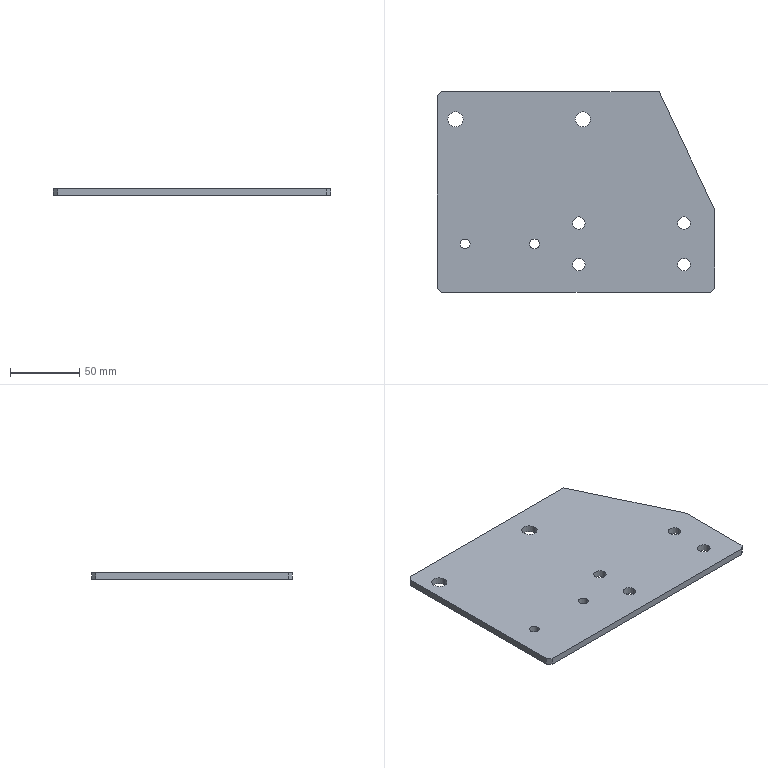Part | SolidWorks | features Extrusion 1 | 1 solid | 26 faces | box 200 x 145 x 5 mm | volume 133825 mm3 | cylinder 16 | plane 10 | commonest cylinder face diameters 9 x8 7 x4 11 x4
STEP:
#1=CARTESIAN_POINT('',(-92.5,52.5,-2.5));
#2=VERTEX_POINT('',#1);
#3=CARTESIAN_POINT('',(-81.5,52.5,-2.5));
#4=VERTEX_POINT('',#3);
#5=CARTESIAN_POINT('',(-87.,52.5,-2.5));
#6=DIRECTION('',(0.,0.,1.));
#7=DIRECTION('',(-1.,0.,0.));
#8=AXIS2_PLACEMENT_3D('',#5,#6,#7);
#9=CIRCLE('',#8,5.5);
#10=EDGE_CURVE('',#2,#4,#9,.T.);
#11=ORIENTED_EDGE('',*,*,#10,.F.);
#12=CARTESIAN_POINT('',(-92.5,52.5,2.5));
#13=VERTEX_POINT('',#12);
#14=CARTESIAN_POINT('',(-92.5,52.5,-2.5));
#15=DIRECTION('',(0.,0.,1.));
#16=VECTOR('',#15,1000.);
#17=LINE('',#14,#16);
#18=EDGE_CURVE('',#2,#13,#17,.T.);
#19=ORIENTED_EDGE('',*,*,#18,.T.);
#20=CARTESIAN_POINT('',(-81.5,52.5,2.5));
#21=VERTEX_POINT('',#20);
#22=CARTESIAN_POINT('',(-87.,52.5,2.5));
#23=DIRECTION('',(0.,0.,1.));
#24=DIRECTION('',(-1.,0.,0.));
#25=AXIS2_PLACEMENT_3D('',#22,#23,#24);
#26=CIRCLE('',#25,5.5);
#27=EDGE_CURVE('',#13,#21,#26,.T.);
#28=ORIENTED_EDGE('',*,*,#27,.T.);
#29=CARTESIAN_POINT('',(-81.5,52.5,-2.5));
#30=DIRECTION('',(0.,0.,1.));
#31=VECTOR('',#30,1000.);
#32=LINE('',#29,#31);
#33=EDGE_CURVE('',#4,#21,#32,.T.);
#34=ORIENTED_EDGE('',*,*,#33,.F.);
#35=EDGE_LOOP('',(#11,#19,#28,#34));
#36=FACE_OUTER_BOUND('',#35,.T.);
#37=CARTESIAN_POINT('',(-87.,52.5,-2.5));
#38=DIRECTION('',(0.,0.,1.));
#39=DIRECTION('',(1.,0.,0.));
#40=AXIS2_PLACEMENT_3D('',#37,#38,#39);
#41=CYLINDRICAL_SURFACE('',#40,5.5);
#42=ADVANCED_FACE('',(#36),#41,.F.);
#43=CARTESIAN_POINT('',(73.5,-22.5,-2.5));
#44=VERTEX_POINT('',#43);
#45=CARTESIAN_POINT('',(82.5,-22.5,-2.5));
#46=VERTEX_POINT('',#45);
#47=CARTESIAN_POINT('',(78.,-22.5,-2.5));
#48=DIRECTION('',(0.,0.,1.));
#49=DIRECTION('',(-1.,0.,0.));
#50=AXIS2_PLACEMENT_3D('',#47,#48,#49);
#51=CIRCLE('',#50,4.5);
#52=EDGE_CURVE('',#44,#46,#51,.T.);
#53=ORIENTED_EDGE('',*,*,#52,.F.);
#54=CARTESIAN_POINT('',(73.5,-22.5,2.5));
#55=VERTEX_POINT('',#54);
#56=CARTESIAN_POINT('',(73.5,-22.5,-2.5));
#57=DIRECTION('',(0.,0.,1.));
#58=VECTOR('',#57,1000.);
#59=LINE('',#56,#58);
#60=EDGE_CURVE('',#44,#55,#59,.T.);
#61=ORIENTED_EDGE('',*,*,#60,.T.);
#62=CARTESIAN_POINT('',(82.5,-22.5,2.5));
#63=VERTEX_POINT('',#62);
#64=CARTESIAN_POINT('',(78.,-22.5,2.5));
#65=DIRECTION('',(0.,0.,1.));
#66=DIRECTION('',(-1.,0.,0.));
#67=AXIS2_PLACEMENT_3D('',#64,#65,#66);
#68=CIRCLE('',#67,4.5);
#69=EDGE_CURVE('',#55,#63,#68,.T.);
#70=ORIENTED_EDGE('',*,*,#69,.T.);
#71=CARTESIAN_POINT('',(82.5,-22.5,-2.5));
#72=DIRECTION('',(0.,0.,1.));
#73=VECTOR('',#72,1000.);
#74=LINE('',#71,#73);
#75=EDGE_CURVE('',#46,#63,#74,.T.);
#76=ORIENTED_EDGE('',*,*,#75,.F.);
#77=EDGE_LOOP('',(#53,#61,#70,#76));
#78=FACE_OUTER_BOUND('',#77,.T.);
#79=CARTESIAN_POINT('',(78.,-22.5,-2.5));
#80=DIRECTION('',(0.,0.,1.));
#81=DIRECTION('',(1.,0.,0.));
#82=AXIS2_PLACEMENT_3D('',#79,#80,#81);
#83=CYLINDRICAL_SURFACE('',#82,4.5);
#84=ADVANCED_FACE('',(#78),#83,.F.);
#85=CARTESIAN_POINT('',(-2.5,-52.5,-2.5));
#86=VERTEX_POINT('',#85);
#87=CARTESIAN_POINT('',(6.5,-52.5,-2.5));
#88=VERTEX_POINT('',#87);
#89=CARTESIAN_POINT('',(2.,-52.5,-2.5));
#90=DIRECTION('',(0.,0.,1.));
#91=DIRECTION('',(-1.,0.,0.));
#92=AXIS2_PLACEMENT_3D('',#89,#90,#91);
#93=CIRCLE('',#92,4.5);
#94=EDGE_CURVE('',#86,#88,#93,.T.);
#95=ORIENTED_EDGE('',*,*,#94,.F.);
#96=CARTESIAN_POINT('',(-2.5,-52.5,2.5));
#97=VERTEX_POINT('',#96);
#98=CARTESIAN_POINT('',(-2.5,-52.5,-2.5));
#99=DIRECTION('',(0.,0.,1.));
#100=VECTOR('',#99,1000.);
#101=LINE('',#98,#100);
#102=EDGE_CURVE('',#86,#97,#101,.T.);
#103=ORIENTED_EDGE('',*,*,#102,.T.);
#104=CARTESIAN_POINT('',(6.5,-52.5,2.5));
#105=VERTEX_POINT('',#104);
#106=CARTESIAN_POINT('',(2.,-52.5,2.5));
#107=DIRECTION('',(0.,0.,1.));
#108=DIRECTION('',(-1.,0.,0.));
#109=AXIS2_PLACEMENT_3D('',#106,#107,#108);
#110=CIRCLE('',#109,4.5);
#111=EDGE_CURVE('',#97,#105,#110,.T.);
#112=ORIENTED_EDGE('',*,*,#111,.T.);
#113=CARTESIAN_POINT('',(6.5,-52.5,-2.5));
#114=DIRECTION('',(0.,0.,1.));
#115=VECTOR('',#114,1000.);
#116=LINE('',#113,#115);
#117=EDGE_CURVE('',#88,#105,#116,.T.);
#118=ORIENTED_EDGE('',*,*,#117,.F.);
#119=EDGE_LOOP('',(#95,#103,#112,#118));
#120=FACE_OUTER_BOUND('',#119,.T.);
#121=CARTESIAN_POINT('',(2.,-52.5,-2.5));
#122=DIRECTION('',(0.,0.,1.));
#123=DIRECTION('',(1.,0.,0.));
#124=AXIS2_PLACEMENT_3D('',#121,#122,#123);
#125=CYLINDRICAL_SURFACE('',#124,4.5);
#126=ADVANCED_FACE('',(#120),#125,.F.);
#127=CARTESIAN_POINT('',(73.5,-52.5,-2.5));
#128=VERTEX_POINT('',#127);
#129=CARTESIAN_POINT('',(82.5,-52.5,-2.5));
#130=VERTEX_POINT('',#129);
#131=CARTESIAN_POINT('',(78.,-52.5,-2.5));
#132=DIRECTION('',(0.,0.,1.));
#133=DIRECTION('',(-1.,0.,0.));
#134=AXIS2_PLACEMENT_3D('',#131,#132,#133);
#135=CIRCLE('',#134,4.5);
#136=EDGE_CURVE('',#128,#130,#135,.T.);
#137=ORIENTED_EDGE('',*,*,#136,.F.);
#138=CARTESIAN_POINT('',(73.5,-52.5,2.5));
#139=VERTEX_POINT('',#138);
#140=CARTESIAN_POINT('',(73.5,-52.5,-2.5));
#141=DIRECTION('',(0.,0.,1.));
#142=VECTOR('',#141,1000.);
#143=LINE('',#140,#142);
#144=EDGE_CURVE('',#128,#139,#143,.T.);
#145=ORIENTED_EDGE('',*,*,#144,.T.);
#146=CARTESIAN_POINT('',(82.5,-52.5,2.5));
#147=VERTEX_POINT('',#146);
#148=CARTESIAN_POINT('',(78.,-52.5,2.5));
#149=DIRECTION('',(0.,0.,1.));
#150=DIRECTION('',(-1.,0.,0.));
#151=AXIS2_PLACEMENT_3D('',#148,#149,#150);
#152=CIRCLE('',#151,4.5);
#153=EDGE_CURVE('',#139,#147,#152,.T.);
#154=ORIENTED_EDGE('',*,*,#153,.T.);
#155=CARTESIAN_POINT('',(82.5,-52.5,-2.5));
#156=DIRECTION('',(0.,0.,1.));
#157=VECTOR('',#156,1000.);
#158=LINE('',#155,#157);
#159=EDGE_CURVE('',#130,#147,#158,.T.);
#160=ORIENTED_EDGE('',*,*,#159,.F.);
#161=EDGE_LOOP('',(#137,#145,#154,#160));
#162=FACE_OUTER_BOUND('',#161,.T.);
#163=CARTESIAN_POINT('',(78.,-52.5,-2.5));
#164=DIRECTION('',(0.,0.,1.));
#165=DIRECTION('',(1.,0.,0.));
#166=AXIS2_PLACEMENT_3D('',#163,#164,#165);
#167=CYLINDRICAL_SURFACE('',#166,4.5);
#168=ADVANCED_FACE('',(#162),#167,.F.);
#169=CARTESIAN_POINT('',(-0.5,52.5,-2.5));
#170=VERTEX_POINT('',#169);
#171=CARTESIAN_POINT('',(10.5,52.5,-2.5));
#172=VERTEX_POINT('',#171);
#173=CARTESIAN_POINT('',(5.,52.5,-2.5));
#174=DIRECTION('',(0.,0.,1.));
#175=DIRECTION('',(-1.,0.,0.));
#176=AXIS2_PLACEMENT_3D('',#173,#174,#175);
#177=CIRCLE('',#176,5.5);
#178=EDGE_CURVE('',#170,#172,#177,.T.);
#179=ORIENTED_EDGE('',*,*,#178,.F.);
#180=CARTESIAN_POINT('',(-0.5,52.5,2.5));
#181=VERTEX_POINT('',#180);
#182=CARTESIAN_POINT('',(-0.5,52.5,-2.5));
#183=DIRECTION('',(0.,0.,1.));
#184=VECTOR('',#183,1000.);
#185=LINE('',#182,#184);
#186=EDGE_CURVE('',#170,#181,#185,.T.);
#187=ORIENTED_EDGE('',*,*,#186,.T.);
#188=CARTESIAN_POINT('',(10.5,52.5,2.5));
#189=VERTEX_POINT('',#188);
#190=CARTESIAN_POINT('',(5.,52.5,2.5));
#191=DIRECTION('',(0.,0.,1.));
#192=DIRECTION('',(-1.,0.,0.));
#193=AXIS2_PLACEMENT_3D('',#190,#191,#192);
#194=CIRCLE('',#193,5.5);
#195=EDGE_CURVE('',#181,#189,#194,.T.);
#196=ORIENTED_EDGE('',*,*,#195,.T.);
#197=CARTESIAN_POINT('',(10.5,52.5,-2.5));
#198=DIRECTION('',(0.,0.,1.));
#199=VECTOR('',#198,1000.);
#200=LINE('',#197,#199);
#201=EDGE_CURVE('',#172,#189,#200,.T.);
#202=ORIENTED_EDGE('',*,*,#201,.F.);
#203=EDGE_LOOP('',(#179,#187,#196,#202));
#204=FACE_OUTER_BOUND('',#203,.T.);
#205=CARTESIAN_POINT('',(5.,52.5,-2.5));
#206=DIRECTION('',(0.,0.,1.));
#207=DIRECTION('',(1.,0.,0.));
#208=AXIS2_PLACEMENT_3D('',#205,#206,#207);
#209=CYLINDRICAL_SURFACE('',#208,5.5);
#210=ADVANCED_FACE('',(#204),#209,.F.);
#211=CARTESIAN_POINT('',(-83.5,-37.5,-2.5));
#212=VERTEX_POINT('',#211);
#213=CARTESIAN_POINT('',(-76.5,-37.5,-2.5));
#214=VERTEX_POINT('',#213);
#215=CARTESIAN_POINT('',(-80.,-37.5,-2.5));
#216=DIRECTION('',(0.,0.,1.));
#217=DIRECTION('',(-1.,0.,0.));
#218=AXIS2_PLACEMENT_3D('',#215,#216,#217);
#219=CIRCLE('',#218,3.5);
#220=EDGE_CURVE('',#212,#214,#219,.T.);
#221=ORIENTED_EDGE('',*,*,#220,.F.);
#222=CARTESIAN_POINT('',(-83.5,-37.5,2.5));
#223=VERTEX_POINT('',#222);
#224=CARTESIAN_POINT('',(-83.5,-37.5,-2.5));
#225=DIRECTION('',(0.,0.,1.));
#226=VECTOR('',#225,1000.);
#227=LINE('',#224,#226);
#228=EDGE_CURVE('',#212,#223,#227,.T.);
#229=ORIENTED_EDGE('',*,*,#228,.T.);
#230=CARTESIAN_POINT('',(-76.5,-37.5,2.5));
#231=VERTEX_POINT('',#230);
#232=CARTESIAN_POINT('',(-80.,-37.5,2.5));
#233=DIRECTION('',(0.,0.,1.));
#234=DIRECTION('',(-1.,0.,0.));
#235=AXIS2_PLACEMENT_3D('',#232,#233,#234);
#236=CIRCLE('',#235,3.5);
#237=EDGE_CURVE('',#223,#231,#236,.T.);
#238=ORIENTED_EDGE('',*,*,#237,.T.);
#239=CARTESIAN_POINT('',(-76.5,-37.5,-2.5));
#240=DIRECTION('',(0.,0.,1.));
#241=VECTOR('',#240,1000.);
#242=LINE('',#239,#241);
#243=EDGE_CURVE('',#214,#231,#242,.T.);
#244=ORIENTED_EDGE('',*,*,#243,.F.);
#245=EDGE_LOOP('',(#221,#229,#238,#244));
#246=FACE_OUTER_BOUND('',#245,.T.);
#247=CARTESIAN_POINT('',(-80.,-37.5,-2.5));
#248=DIRECTION('',(0.,0.,1.));
#249=DIRECTION('',(1.,0.,0.));
#250=AXIS2_PLACEMENT_3D('',#247,#248,#249);
#251=CYLINDRICAL_SURFACE('',#250,3.5);
#252=ADVANCED_FACE('',(#246),#251,.F.);
#253=CARTESIAN_POINT('',(-33.5,-37.5,-2.5));
#254=VERTEX_POINT('',#253);
#255=CARTESIAN_POINT('',(-26.5,-37.5,-2.5));
#256=VERTEX_POINT('',#255);
#257=CARTESIAN_POINT('',(-30.,-37.5,-2.5));
#258=DIRECTION('',(0.,0.,1.));
#259=DIRECTION('',(-1.,0.,0.));
#260=AXIS2_PLACEMENT_3D('',#257,#258,#259);
#261=CIRCLE('',#260,3.5);
#262=EDGE_CURVE('',#254,#256,#261,.T.);
#263=ORIENTED_EDGE('',*,*,#262,.F.);
#264=CARTESIAN_POINT('',(-33.5,-37.5,2.5));
#265=VERTEX_POINT('',#264);
#266=CARTESIAN_POINT('',(-33.5,-37.5,-2.5));
#267=DIRECTION('',(0.,0.,1.));
#268=VECTOR('',#267,1000.);
#269=LINE('',#266,#268);
#270=EDGE_CURVE('',#254,#265,#269,.T.);
#271=ORIENTED_EDGE('',*,*,#270,.T.);
#272=CARTESIAN_POINT('',(-26.5,-37.5,2.5));
#273=VERTEX_POINT('',#272);
#274=CARTESIAN_POINT('',(-30.,-37.5,2.5));
#275=DIRECTION('',(0.,0.,1.));
#276=DIRECTION('',(-1.,0.,0.));
#277=AXIS2_PLACEMENT_3D('',#274,#275,#276);
#278=CIRCLE('',#277,3.5);
#279=EDGE_CURVE('',#265,#273,#278,.T.);
#280=ORIENTED_EDGE('',*,*,#279,.T.);
#281=CARTESIAN_POINT('',(-26.5,-37.5,-2.5));
#282=DIRECTION('',(0.,0.,1.));
#283=VECTOR('',#282,1000.);
#284=LINE('',#281,#283);
#285=EDGE_CURVE('',#256,#273,#284,.T.);
#286=ORIENTED_EDGE('',*,*,#285,.F.);
#287=EDGE_LOOP('',(#263,#271,#280,#286));
#288=FACE_OUTER_BOUND('',#287,.T.);
#289=CARTESIAN_POINT('',(-30.,-37.5,-2.5));
#290=DIRECTION('',(0.,0.,1.));
#291=DIRECTION('',(1.,0.,0.));
#292=AXIS2_PLACEMENT_3D('',#289,#290,#291);
#293=CYLINDRICAL_SURFACE('',#292,3.5);
#294=ADVANCED_FACE('',(#288),#293,.F.);
#295=CARTESIAN_POINT('',(-2.5,-22.5,-2.5));
#296=VERTEX_POINT('',#295);
#297=CARTESIAN_POINT('',(6.5,-22.5,-2.5));
#298=VERTEX_POINT('',#297);
#299=CARTESIAN_POINT('',(2.,-22.5,-2.5));
#300=DIRECTION('',(0.,0.,1.));
#301=DIRECTION('',(-1.,0.,0.));
#302=AXIS2_PLACEMENT_3D('',#299,#300,#301);
#303=CIRCLE('',#302,4.5);
#304=EDGE_CURVE('',#296,#298,#303,.T.);
#305=ORIENTED_EDGE('',*,*,#304,.F.);
#306=CARTESIAN_POINT('',(-2.5,-22.5,2.5));
#307=VERTEX_POINT('',#306);
#308=CARTESIAN_POINT('',(-2.5,-22.5,-2.5));
#309=DIRECTION('',(0.,0.,1.));
#310=VECTOR('',#309,1000.);
#311=LINE('',#308,#310);
#312=EDGE_CURVE('',#296,#307,#311,.T.);
#313=ORIENTED_EDGE('',*,*,#312,.T.);
#314=CARTESIAN_POINT('',(6.5,-22.5,2.5));
#315=VERTEX_POINT('',#314);
#316=CARTESIAN_POINT('',(2.,-22.5,2.5));
#317=DIRECTION('',(0.,0.,1.));
#318=DIRECTION('',(-1.,0.,0.));
#319=AXIS2_PLACEMENT_3D('',#316,#317,#318);
#320=CIRCLE('',#319,4.5);
#321=EDGE_CURVE('',#307,#315,#320,.T.);
#322=ORIENTED_EDGE('',*,*,#321,.T.);
#323=CARTESIAN_POINT('',(6.5,-22.5,-2.5));
#324=DIRECTION('',(0.,0.,1.));
#325=VECTOR('',#324,1000.);
#326=LINE('',#323,#325);
#327=EDGE_CURVE('',#298,#315,#326,.T.);
#328=ORIENTED_EDGE('',*,*,#327,.F.);
#329=EDGE_LOOP('',(#305,#313,#322,#328));
#330=FACE_OUTER_BOUND('',#329,.T.);
#331=CARTESIAN_POINT('',(2.,-22.5,-2.5));
#332=DIRECTION('',(0.,0.,1.));
#333=DIRECTION('',(1.,0.,0.));
#334=AXIS2_PLACEMENT_3D('',#331,#332,#333);
#335=CYLINDRICAL_SURFACE('',#334,4.5);
#336=ADVANCED_FACE('',(#330),#335,.F.);
#337=CARTESIAN_POINT('',(-100.,-69.5,2.5));
#338=VERTEX_POINT('',#337);
#339=CARTESIAN_POINT('',(-97.,-72.5,2.5));
#340=VERTEX_POINT('',#339);
#341=CARTESIAN_POINT('',(-100.,-69.5,2.5));
#342=DIRECTION('',(0.7071,-0.7071,0.));
#343=VECTOR('',#342,1000.);
#344=LINE('',#341,#343);
#345=EDGE_CURVE('',#338,#340,#344,.T.);
#346=ORIENTED_EDGE('',*,*,#345,.F.);
#347=CARTESIAN_POINT('',(-100.,-69.5,-2.5));
#348=VERTEX_POINT('',#347);
#349=CARTESIAN_POINT('',(-100.,-69.5,-2.5));
#350=DIRECTION('',(0.,0.,1.));
#351=VECTOR('',#350,1000.);
#352=LINE('',#349,#351);
#353=EDGE_CURVE('',#348,#338,#352,.T.);
#354=ORIENTED_EDGE('',*,*,#353,.F.);
#355=CARTESIAN_POINT('',(-97.,-72.5,-2.5));
#356=VERTEX_POINT('',#355);
#357=CARTESIAN_POINT('',(-100.,-69.5,-2.5));
#358=DIRECTION('',(0.7071,-0.7071,0.));
#359=VECTOR('',#358,1000.);
#360=LINE('',#357,#359);
#361=EDGE_CURVE('',#348,#356,#360,.T.);
#362=ORIENTED_EDGE('',*,*,#361,.T.);
#363=CARTESIAN_POINT('',(-97.,-72.5,-2.5));
#364=DIRECTION('',(0.,0.,1.));
#365=VECTOR('',#364,1000.);
#366=LINE('',#363,#365);
#367=EDGE_CURVE('',#356,#340,#366,.T.);
#368=ORIENTED_EDGE('',*,*,#367,.T.);
#369=EDGE_LOOP('',(#346,#354,#362,#368));
#370=FACE_OUTER_BOUND('',#369,.T.);
#371=CARTESIAN_POINT('',(-100.,-69.5,-2.5));
#372=DIRECTION('',(-0.7071,-0.7071,0.));
#373=DIRECTION('',(0.7071,-0.7071,0.));
#374=AXIS2_PLACEMENT_3D('',#371,#372,#373);
#375=PLANE('',#374);
#376=ADVANCED_FACE('',(#370),#375,.T.);
#377=CARTESIAN_POINT('',(-100.,69.5,2.5));
#378=VERTEX_POINT('',#377);
#379=CARTESIAN_POINT('',(-100.,69.5,2.5));
#380=DIRECTION('',(0.,-1.,0.));
#381=VECTOR('',#380,1000.);
#382=LINE('',#379,#381);
#383=EDGE_CURVE('',#378,#338,#382,.T.);
#384=ORIENTED_EDGE('',*,*,#383,.F.);
#385=CARTESIAN_POINT('',(-100.,69.5,-2.5));
#386=VERTEX_POINT('',#385);
#387=CARTESIAN_POINT('',(-100.,69.5,-2.5));
#388=DIRECTION('',(0.,0.,1.));
#389=VECTOR('',#388,1000.);
#390=LINE('',#387,#389);
#391=EDGE_CURVE('',#386,#378,#390,.T.);
#392=ORIENTED_EDGE('',*,*,#391,.F.);
#393=CARTESIAN_POINT('',(-100.,69.5,-2.5));
#394=DIRECTION('',(0.,-1.,0.));
#395=VECTOR('',#394,1000.);
#396=LINE('',#393,#395);
#397=EDGE_CURVE('',#386,#348,#396,.T.);
#398=ORIENTED_EDGE('',*,*,#397,.T.);
#399=ORIENTED_EDGE('',*,*,#353,.T.);
#400=EDGE_LOOP('',(#384,#392,#398,#399));
#401=FACE_OUTER_BOUND('',#400,.T.);
#402=CARTESIAN_POINT('',(-100.,69.5,-2.5));
#403=DIRECTION('',(-1.,0.,0.));
#404=DIRECTION('',(0.,0.,1.));
#405=AXIS2_PLACEMENT_3D('',#402,#403,#404);
#406=PLANE('',#405);
#407=ADVANCED_FACE('',(#401),#406,.T.);
#408=CARTESIAN_POINT('',(-97.,72.5,2.5));
#409=VERTEX_POINT('',#408);
#410=CARTESIAN_POINT('',(-97.,72.5,2.5));
#411=DIRECTION('',(-0.7071,-0.7071,0.));
#412=VECTOR('',#411,1000.);
#413=LINE('',#410,#412);
#414=EDGE_CURVE('',#409,#378,#413,.T.);
#415=ORIENTED_EDGE('',*,*,#414,.F.);
#416=CARTESIAN_POINT('',(-97.,72.5,-2.5));
#417=VERTEX_POINT('',#416);
#418=CARTESIAN_POINT('',(-97.,72.5,-2.5));
#419=DIRECTION('',(0.,0.,1.));
#420=VECTOR('',#419,1000.);
#421=LINE('',#418,#420);
#422=EDGE_CURVE('',#417,#409,#421,.T.);
#423=ORIENTED_EDGE('',*,*,#422,.F.);
#424=CARTESIAN_POINT('',(-97.,72.5,-2.5));
#425=DIRECTION('',(-0.7071,-0.7071,0.));
#426=VECTOR('',#425,1000.);
#427=LINE('',#424,#426);
#428=EDGE_CURVE('',#417,#386,#427,.T.);
#429=ORIENTED_EDGE('',*,*,#428,.T.);
#430=ORIENTED_EDGE('',*,*,#391,.T.);
#431=EDGE_LOOP('',(#415,#423,#429,#430));
#432=FACE_OUTER_BOUND('',#431,.T.);
#433=CARTESIAN_POINT('',(-97.,72.5,-2.5));
#434=DIRECTION('',(-0.7071,0.7071,0.));
#435=DIRECTION('',(-0.7071,-0.7071,0.));
#436=AXIS2_PLACEMENT_3D('',#433,#434,#435);
#437=PLANE('',#436);
#438=ADVANCED_FACE('',(#432),#437,.T.);
#439=CARTESIAN_POINT('',(60.,72.5,2.5));
#440=VERTEX_POINT('',#439);
#441=CARTESIAN_POINT('',(60.,72.5,2.5));
#442=DIRECTION('',(-1.,0.,0.));
#443=VECTOR('',#442,1000.);
#444=LINE('',#441,#443);
#445=EDGE_CURVE('',#440,#409,#444,.T.);
#446=ORIENTED_EDGE('',*,*,#445,.F.);
#447=CARTESIAN_POINT('',(60.,72.5,-2.5));
#448=VERTEX_POINT('',#447);
#449=CARTESIAN_POINT('',(60.,72.5,-2.5));
#450=DIRECTION('',(0.,0.,1.));
#451=VECTOR('',#450,1000.);
#452=LINE('',#449,#451);
#453=EDGE_CURVE('',#448,#440,#452,.T.);
#454=ORIENTED_EDGE('',*,*,#453,.F.);
#455=CARTESIAN_POINT('',(60.,72.5,-2.5));
#456=DIRECTION('',(-1.,0.,0.));
#457=VECTOR('',#456,1000.);
#458=LINE('',#455,#457);
#459=EDGE_CURVE('',#448,#417,#458,.T.);
#460=ORIENTED_EDGE('',*,*,#459,.T.);
#461=ORIENTED_EDGE('',*,*,#422,.T.);
#462=EDGE_LOOP('',(#446,#454,#460,#461));
#463=FACE_OUTER_BOUND('',#462,.T.);
#464=CARTESIAN_POINT('',(60.,72.5,-2.5));
#465=DIRECTION('',(0.,1.,0.));
#466=DIRECTION('',(0.,0.,1.));
#467=AXIS2_PLACEMENT_3D('',#464,#465,#466);
#468=PLANE('',#467);
#469=ADVANCED_FACE('',(#463),#468,.T.);
#470=CARTESIAN_POINT('',(100.,-12.5,2.5));
#471=VERTEX_POINT('',#470);
#472=CARTESIAN_POINT('',(100.,-12.5,2.5));
#473=DIRECTION('',(-0.4258,0.9048,0.));
#474=VECTOR('',#473,1000.);
#475=LINE('',#472,#474);
#476=EDGE_CURVE('',#471,#440,#475,.T.);
#477=ORIENTED_EDGE('',*,*,#476,.F.);
#478=CARTESIAN_POINT('',(100.,-12.5,-2.5));
#479=VERTEX_POINT('',#478);
#480=CARTESIAN_POINT('',(100.,-12.5,-2.5));
#481=DIRECTION('',(0.,0.,1.));
#482=VECTOR('',#481,1000.);
#483=LINE('',#480,#482);
#484=EDGE_CURVE('',#479,#471,#483,.T.);
#485=ORIENTED_EDGE('',*,*,#484,.F.);
#486=CARTESIAN_POINT('',(100.,-12.5,-2.5));
#487=DIRECTION('',(-0.4258,0.9048,0.));
#488=VECTOR('',#487,1000.);
#489=LINE('',#486,#488);
#490=EDGE_CURVE('',#479,#448,#489,.T.);
#491=ORIENTED_EDGE('',*,*,#490,.T.);
#492=ORIENTED_EDGE('',*,*,#453,.T.);
#493=EDGE_LOOP('',(#477,#485,#491,#492));
#494=FACE_OUTER_BOUND('',#493,.T.);
#495=CARTESIAN_POINT('',(100.,-12.5,-2.5));
#496=DIRECTION('',(0.9048,0.4258,0.));
#497=DIRECTION('',(-0.4258,0.9048,0.));
#498=AXIS2_PLACEMENT_3D('',#495,#496,#497);
#499=PLANE('',#498);
#500=ADVANCED_FACE('',(#494),#499,.T.);
#501=CARTESIAN_POINT('',(100.,-69.5,2.5));
#502=VERTEX_POINT('',#501);
#503=CARTESIAN_POINT('',(100.,-69.5,2.5));
#504=DIRECTION('',(0.,1.,0.));
#505=VECTOR('',#504,1000.);
#506=LINE('',#503,#505);
#507=EDGE_CURVE('',#502,#471,#506,.T.);
#508=ORIENTED_EDGE('',*,*,#507,.F.);
#509=CARTESIAN_POINT('',(100.,-69.5,-2.5));
#510=VERTEX_POINT('',#509);
#511=CARTESIAN_POINT('',(100.,-69.5,-2.5));
#512=DIRECTION('',(0.,0.,1.));
#513=VECTOR('',#512,1000.);
#514=LINE('',#511,#513);
#515=EDGE_CURVE('',#510,#502,#514,.T.);
#516=ORIENTED_EDGE('',*,*,#515,.F.);
#517=CARTESIAN_POINT('',(100.,-69.5,-2.5));
#518=DIRECTION('',(0.,1.,0.));
#519=VECTOR('',#518,1000.);
#520=LINE('',#517,#519);
#521=EDGE_CURVE('',#510,#479,#520,.T.);
#522=ORIENTED_EDGE('',*,*,#521,.T.);
#523=ORIENTED_EDGE('',*,*,#484,.T.);
#524=EDGE_LOOP('',(#508,#516,#522,#523));
#525=FACE_OUTER_BOUND('',#524,.T.);
#526=CARTESIAN_POINT('',(100.,-69.5,-2.5));
#527=DIRECTION('',(1.,0.,0.));
#528=DIRECTION('',(0.,0.,-1.));
#529=AXIS2_PLACEMENT_3D('',#526,#527,#528);
#530=PLANE('',#529);
#531=ADVANCED_FACE('',(#525),#530,.T.);
#532=CARTESIAN_POINT('',(97.,-72.5,2.5));
#533=VERTEX_POINT('',#532);
#534=CARTESIAN_POINT('',(97.,-72.5,2.5));
#535=DIRECTION('',(0.7071,0.7071,0.));
#536=VECTOR('',#535,1000.);
#537=LINE('',#534,#536);
#538=EDGE_CURVE('',#533,#502,#537,.T.);
#539=ORIENTED_EDGE('',*,*,#538,.F.);
#540=CARTESIAN_POINT('',(97.,-72.5,-2.5));
#541=VERTEX_POINT('',#540);
#542=CARTESIAN_POINT('',(97.,-72.5,-2.5));
#543=DIRECTION('',(0.,0.,1.));
#544=VECTOR('',#543,1000.);
#545=LINE('',#542,#544);
#546=EDGE_CURVE('',#541,#533,#545,.T.);
#547=ORIENTED_EDGE('',*,*,#546,.F.);
#548=CARTESIAN_POINT('',(97.,-72.5,-2.5));
#549=DIRECTION('',(0.7071,0.7071,0.));
#550=VECTOR('',#549,1000.);
#551=LINE('',#548,#550);
#552=EDGE_CURVE('',#541,#510,#551,.T.);
#553=ORIENTED_EDGE('',*,*,#552,.T.);
#554=ORIENTED_EDGE('',*,*,#515,.T.);
#555=EDGE_LOOP('',(#539,#547,#553,#554));
#556=FACE_OUTER_BOUND('',#555,.T.);
#557=CARTESIAN_POINT('',(97.,-72.5,-2.5));
#558=DIRECTION('',(0.7071,-0.7071,0.));
#559=DIRECTION('',(0.7071,0.7071,0.));
#560=AXIS2_PLACEMENT_3D('',#557,#558,#559);
#561=PLANE('',#560);
#562=ADVANCED_FACE('',(#556),#561,.T.);
#563=CARTESIAN_POINT('',(-97.,-72.5,2.5));
#564=DIRECTION('',(1.,0.,0.));
#565=VECTOR('',#564,1000.);
#566=LINE('',#563,#565);
#567=EDGE_CURVE('',#340,#533,#566,.T.);
#568=ORIENTED_EDGE('',*,*,#567,.F.);
#569=ORIENTED_EDGE('',*,*,#367,.F.);
#570=CARTESIAN_POINT('',(-97.,-72.5,-2.5));
#571=DIRECTION('',(1.,0.,0.));
#572=VECTOR('',#571,1000.);
#573=LINE('',#570,#572);
#574=EDGE_CURVE('',#356,#541,#573,.T.);
#575=ORIENTED_EDGE('',*,*,#574,.T.);
#576=ORIENTED_EDGE('',*,*,#546,.T.);
#577=EDGE_LOOP('',(#568,#569,#575,#576));
#578=FACE_OUTER_BOUND('',#577,.T.);
#579=CARTESIAN_POINT('',(-97.,-72.5,-2.5));
#580=DIRECTION('',(0.,-1.,0.));
#581=DIRECTION('',(0.,0.,-1.));
#582=AXIS2_PLACEMENT_3D('',#579,#580,#581);
#583=PLANE('',#582);
#584=ADVANCED_FACE('',(#578),#583,.T.);
#585=CARTESIAN_POINT('',(-87.,52.5,-2.5));
#586=DIRECTION('',(0.,0.,1.));
#587=DIRECTION('',(-1.,0.,0.));
#588=AXIS2_PLACEMENT_3D('',#585,#586,#587);
#589=CIRCLE('',#588,5.5);
#590=EDGE_CURVE('',#4,#2,#589,.T.);
#591=ORIENTED_EDGE('',*,*,#590,.T.);
#592=ORIENTED_EDGE('',*,*,#10,.T.);
#593=EDGE_LOOP('',(#591,#592));
#594=FACE_BOUND('',#593,.T.);
#595=CARTESIAN_POINT('',(78.,-22.5,-2.5));
#596=DIRECTION('',(0.,0.,1.));
#597=DIRECTION('',(-1.,0.,0.));
#598=AXIS2_PLACEMENT_3D('',#595,#596,#597);
#599=CIRCLE('',#598,4.5);
#600=EDGE_CURVE('',#46,#44,#599,.T.);
#601=ORIENTED_EDGE('',*,*,#600,.T.);
#602=ORIENTED_EDGE('',*,*,#52,.T.);
#603=EDGE_LOOP('',(#601,#602));
#604=FACE_BOUND('',#603,.T.);
#605=CARTESIAN_POINT('',(2.,-52.5,-2.5));
#606=DIRECTION('',(0.,0.,1.));
#607=DIRECTION('',(-1.,0.,0.));
#608=AXIS2_PLACEMENT_3D('',#605,#606,#607);
#609=CIRCLE('',#608,4.5);
#610=EDGE_CURVE('',#88,#86,#609,.T.);
#611=ORIENTED_EDGE('',*,*,#610,.T.);
#612=ORIENTED_EDGE('',*,*,#94,.T.);
#613=EDGE_LOOP('',(#611,#612));
#614=FACE_BOUND('',#613,.T.);
#615=CARTESIAN_POINT('',(78.,-52.5,-2.5));
#616=DIRECTION('',(0.,0.,1.));
#617=DIRECTION('',(-1.,0.,0.));
#618=AXIS2_PLACEMENT_3D('',#615,#616,#617);
#619=CIRCLE('',#618,4.5);
#620=EDGE_CURVE('',#130,#128,#619,.T.);
#621=ORIENTED_EDGE('',*,*,#620,.T.);
#622=ORIENTED_EDGE('',*,*,#136,.T.);
#623=EDGE_LOOP('',(#621,#622));
#624=FACE_BOUND('',#623,.T.);
#625=CARTESIAN_POINT('',(5.,52.5,-2.5));
#626=DIRECTION('',(0.,0.,1.));
#627=DIRECTION('',(-1.,0.,0.));
#628=AXIS2_PLACEMENT_3D('',#625,#626,#627);
#629=CIRCLE('',#628,5.5);
#630=EDGE_CURVE('',#172,#170,#629,.T.);
#631=ORIENTED_EDGE('',*,*,#630,.T.);
#632=ORIENTED_EDGE('',*,*,#178,.T.);
#633=EDGE_LOOP('',(#631,#632));
#634=FACE_BOUND('',#633,.T.);
#635=CARTESIAN_POINT('',(-80.,-37.5,-2.5));
#636=DIRECTION('',(0.,0.,1.));
#637=DIRECTION('',(-1.,0.,0.));
#638=AXIS2_PLACEMENT_3D('',#635,#636,#637);
#639=CIRCLE('',#638,3.5);
#640=EDGE_CURVE('',#214,#212,#639,.T.);
#641=ORIENTED_EDGE('',*,*,#640,.T.);
#642=ORIENTED_EDGE('',*,*,#220,.T.);
#643=EDGE_LOOP('',(#641,#642));
#644=FACE_BOUND('',#643,.T.);
#645=CARTESIAN_POINT('',(-30.,-37.5,-2.5));
#646=DIRECTION('',(0.,0.,1.));
#647=DIRECTION('',(-1.,0.,0.));
#648=AXIS2_PLACEMENT_3D('',#645,#646,#647);
#649=CIRCLE('',#648,3.5);
#650=EDGE_CURVE('',#256,#254,#649,.T.);
#651=ORIENTED_EDGE('',*,*,#650,.T.);
#652=ORIENTED_EDGE('',*,*,#262,.T.);
#653=EDGE_LOOP('',(#651,#652));
#654=FACE_BOUND('',#653,.T.);
#655=CARTESIAN_POINT('',(2.,-22.5,-2.5));
#656=DIRECTION('',(0.,0.,1.));
#657=DIRECTION('',(-1.,0.,0.));
#658=AXIS2_PLACEMENT_3D('',#655,#656,#657);
#659=CIRCLE('',#658,4.5);
#660=EDGE_CURVE('',#298,#296,#659,.T.);
#661=ORIENTED_EDGE('',*,*,#660,.T.);
#662=ORIENTED_EDGE('',*,*,#304,.T.);
#663=EDGE_LOOP('',(#661,#662));
#664=FACE_BOUND('',#663,.T.);
#665=ORIENTED_EDGE('',*,*,#361,.F.);
#666=ORIENTED_EDGE('',*,*,#397,.F.);
#667=ORIENTED_EDGE('',*,*,#428,.F.);
#668=ORIENTED_EDGE('',*,*,#459,.F.);
#669=ORIENTED_EDGE('',*,*,#490,.F.);
#670=ORIENTED_EDGE('',*,*,#521,.F.);
#671=ORIENTED_EDGE('',*,*,#552,.F.);
#672=ORIENTED_EDGE('',*,*,#574,.F.);
#673=EDGE_LOOP('',(#665,#666,#667,#668,#669,#670,#671,#672));
#674=FACE_OUTER_BOUND('',#673,.T.);
#675=CARTESIAN_POINT('',(0.,0.,-2.5));
#676=DIRECTION('',(0.,0.,1.));
#677=DIRECTION('',(1.,0.,0.));
#678=AXIS2_PLACEMENT_3D('',#675,#676,#677);
#679=PLANE('',#678);
#680=ADVANCED_FACE('',(#594,#604,#614,#624,#634,#644,#654,#664,#674),#679,.F.);
#681=CARTESIAN_POINT('',(-87.,52.5,2.5));
#682=DIRECTION('',(0.,0.,1.));
#683=DIRECTION('',(-1.,0.,0.));
#684=AXIS2_PLACEMENT_3D('',#681,#682,#683);
#685=CIRCLE('',#684,5.5);
#686=EDGE_CURVE('',#21,#13,#685,.T.);
#687=ORIENTED_EDGE('',*,*,#686,.F.);
#688=ORIENTED_EDGE('',*,*,#27,.F.);
#689=EDGE_LOOP('',(#687,#688));
#690=FACE_BOUND('',#689,.T.);
#691=CARTESIAN_POINT('',(78.,-22.5,2.5));
#692=DIRECTION('',(0.,0.,1.));
#693=DIRECTION('',(-1.,0.,0.));
#694=AXIS2_PLACEMENT_3D('',#691,#692,#693);
#695=CIRCLE('',#694,4.5);
#696=EDGE_CURVE('',#63,#55,#695,.T.);
#697=ORIENTED_EDGE('',*,*,#696,.F.);
#698=ORIENTED_EDGE('',*,*,#69,.F.);
#699=EDGE_LOOP('',(#697,#698));
#700=FACE_BOUND('',#699,.T.);
#701=CARTESIAN_POINT('',(2.,-52.5,2.5));
#702=DIRECTION('',(0.,0.,1.));
#703=DIRECTION('',(-1.,0.,0.));
#704=AXIS2_PLACEMENT_3D('',#701,#702,#703);
#705=CIRCLE('',#704,4.5);
#706=EDGE_CURVE('',#105,#97,#705,.T.);
#707=ORIENTED_EDGE('',*,*,#706,.F.);
#708=ORIENTED_EDGE('',*,*,#111,.F.);
#709=EDGE_LOOP('',(#707,#708));
#710=FACE_BOUND('',#709,.T.);
#711=CARTESIAN_POINT('',(78.,-52.5,2.5));
#712=DIRECTION('',(0.,0.,1.));
#713=DIRECTION('',(-1.,0.,0.));
#714=AXIS2_PLACEMENT_3D('',#711,#712,#713);
#715=CIRCLE('',#714,4.5);
#716=EDGE_CURVE('',#147,#139,#715,.T.);
#717=ORIENTED_EDGE('',*,*,#716,.F.);
#718=ORIENTED_EDGE('',*,*,#153,.F.);
#719=EDGE_LOOP('',(#717,#718));
#720=FACE_BOUND('',#719,.T.);
#721=CARTESIAN_POINT('',(5.,52.5,2.5));
#722=DIRECTION('',(0.,0.,1.));
#723=DIRECTION('',(-1.,0.,0.));
#724=AXIS2_PLACEMENT_3D('',#721,#722,#723);
#725=CIRCLE('',#724,5.5);
#726=EDGE_CURVE('',#189,#181,#725,.T.);
#727=ORIENTED_EDGE('',*,*,#726,.F.);
#728=ORIENTED_EDGE('',*,*,#195,.F.);
#729=EDGE_LOOP('',(#727,#728));
#730=FACE_BOUND('',#729,.T.);
#731=CARTESIAN_POINT('',(-80.,-37.5,2.5));
#732=DIRECTION('',(0.,0.,1.));
#733=DIRECTION('',(-1.,0.,0.));
#734=AXIS2_PLACEMENT_3D('',#731,#732,#733);
#735=CIRCLE('',#734,3.5);
#736=EDGE_CURVE('',#231,#223,#735,.T.);
#737=ORIENTED_EDGE('',*,*,#736,.F.);
#738=ORIENTED_EDGE('',*,*,#237,.F.);
#739=EDGE_LOOP('',(#737,#738));
#740=FACE_BOUND('',#739,.T.);
#741=CARTESIAN_POINT('',(-30.,-37.5,2.5));
#742=DIRECTION('',(0.,0.,1.));
#743=DIRECTION('',(-1.,0.,0.));
#744=AXIS2_PLACEMENT_3D('',#741,#742,#743);
#745=CIRCLE('',#744,3.5);
#746=EDGE_CURVE('',#273,#265,#745,.T.);
#747=ORIENTED_EDGE('',*,*,#746,.F.);
#748=ORIENTED_EDGE('',*,*,#279,.F.);
#749=EDGE_LOOP('',(#747,#748));
#750=FACE_BOUND('',#749,.T.);
#751=CARTESIAN_POINT('',(2.,-22.5,2.5));
#752=DIRECTION('',(0.,0.,1.));
#753=DIRECTION('',(-1.,0.,0.));
#754=AXIS2_PLACEMENT_3D('',#751,#752,#753);
#755=CIRCLE('',#754,4.5);
#756=EDGE_CURVE('',#315,#307,#755,.T.);
#757=ORIENTED_EDGE('',*,*,#756,.F.);
#758=ORIENTED_EDGE('',*,*,#321,.F.);
#759=EDGE_LOOP('',(#757,#758));
#760=FACE_BOUND('',#759,.T.);
#761=ORIENTED_EDGE('',*,*,#345,.T.);
#762=ORIENTED_EDGE('',*,*,#567,.T.);
#763=ORIENTED_EDGE('',*,*,#538,.T.);
#764=ORIENTED_EDGE('',*,*,#507,.T.);
#765=ORIENTED_EDGE('',*,*,#476,.T.);
#766=ORIENTED_EDGE('',*,*,#445,.T.);
#767=ORIENTED_EDGE('',*,*,#414,.T.);
#768=ORIENTED_EDGE('',*,*,#383,.T.);
#769=EDGE_LOOP('',(#761,#762,#763,#764,#765,#766,#767,#768));
#770=FACE_OUTER_BOUND('',#769,.T.);
#771=CARTESIAN_POINT('',(0.,0.,2.5));
#772=DIRECTION('',(0.,0.,1.));
#773=DIRECTION('',(1.,0.,0.));
#774=AXIS2_PLACEMENT_3D('',#771,#772,#773);
#775=PLANE('',#774);
#776=ADVANCED_FACE('',(#690,#700,#710,#720,#730,#740,#750,#760,#770),#775,.T.);
#777=ORIENTED_EDGE('',*,*,#312,.F.);
#778=ORIENTED_EDGE('',*,*,#660,.F.);
#779=ORIENTED_EDGE('',*,*,#327,.T.);
#780=ORIENTED_EDGE('',*,*,#756,.T.);
#781=EDGE_LOOP('',(#777,#778,#779,#780));
#782=FACE_OUTER_BOUND('',#781,.T.);
#783=CARTESIAN_POINT('',(2.,-22.5,-2.5));
#784=DIRECTION('',(0.,0.,1.));
#785=DIRECTION('',(1.,0.,0.));
#786=AXIS2_PLACEMENT_3D('',#783,#784,#785);
#787=CYLINDRICAL_SURFACE('',#786,4.5);
#788=ADVANCED_FACE('',(#782),#787,.F.);
#789=ORIENTED_EDGE('',*,*,#270,.F.);
#790=ORIENTED_EDGE('',*,*,#650,.F.);
#791=ORIENTED_EDGE('',*,*,#285,.T.);
#792=ORIENTED_EDGE('',*,*,#746,.T.);
#793=EDGE_LOOP('',(#789,#790,#791,#792));
#794=FACE_OUTER_BOUND('',#793,.T.);
#795=CARTESIAN_POINT('',(-30.,-37.5,-2.5));
#796=DIRECTION('',(0.,0.,1.));
#797=DIRECTION('',(1.,0.,0.));
#798=AXIS2_PLACEMENT_3D('',#795,#796,#797);
#799=CYLINDRICAL_SURFACE('',#798,3.5);
#800=ADVANCED_FACE('',(#794),#799,.F.);
#801=ORIENTED_EDGE('',*,*,#228,.F.);
#802=ORIENTED_EDGE('',*,*,#640,.F.);
#803=ORIENTED_EDGE('',*,*,#243,.T.);
#804=ORIENTED_EDGE('',*,*,#736,.T.);
#805=EDGE_LOOP('',(#801,#802,#803,#804));
#806=FACE_OUTER_BOUND('',#805,.T.);
#807=CARTESIAN_POINT('',(-80.,-37.5,-2.5));
#808=DIRECTION('',(0.,0.,1.));
#809=DIRECTION('',(1.,0.,0.));
#810=AXIS2_PLACEMENT_3D('',#807,#808,#809);
#811=CYLINDRICAL_SURFACE('',#810,3.5);
#812=ADVANCED_FACE('',(#806),#811,.F.);
#813=ORIENTED_EDGE('',*,*,#186,.F.);
#814=ORIENTED_EDGE('',*,*,#630,.F.);
#815=ORIENTED_EDGE('',*,*,#201,.T.);
#816=ORIENTED_EDGE('',*,*,#726,.T.);
#817=EDGE_LOOP('',(#813,#814,#815,#816));
#818=FACE_OUTER_BOUND('',#817,.T.);
#819=CARTESIAN_POINT('',(5.,52.5,-2.5));
#820=DIRECTION('',(0.,0.,1.));
#821=DIRECTION('',(1.,0.,0.));
#822=AXIS2_PLACEMENT_3D('',#819,#820,#821);
#823=CYLINDRICAL_SURFACE('',#822,5.5);
#824=ADVANCED_FACE('',(#818),#823,.F.);
#825=ORIENTED_EDGE('',*,*,#144,.F.);
#826=ORIENTED_EDGE('',*,*,#620,.F.);
#827=ORIENTED_EDGE('',*,*,#159,.T.);
#828=ORIENTED_EDGE('',*,*,#716,.T.);
#829=EDGE_LOOP('',(#825,#826,#827,#828));
#830=FACE_OUTER_BOUND('',#829,.T.);
#831=CARTESIAN_POINT('',(78.,-52.5,-2.5));
#832=DIRECTION('',(0.,0.,1.));
#833=DIRECTION('',(1.,0.,0.));
#834=AXIS2_PLACEMENT_3D('',#831,#832,#833);
#835=CYLINDRICAL_SURFACE('',#834,4.5);
#836=ADVANCED_FACE('',(#830),#835,.F.);
#837=ORIENTED_EDGE('',*,*,#102,.F.);
#838=ORIENTED_EDGE('',*,*,#610,.F.);
#839=ORIENTED_EDGE('',*,*,#117,.T.);
#840=ORIENTED_EDGE('',*,*,#706,.T.);
#841=EDGE_LOOP('',(#837,#838,#839,#840));
#842=FACE_OUTER_BOUND('',#841,.T.);
#843=CARTESIAN_POINT('',(2.,-52.5,-2.5));
#844=DIRECTION('',(0.,0.,1.));
#845=DIRECTION('',(1.,0.,0.));
#846=AXIS2_PLACEMENT_3D('',#843,#844,#845);
#847=CYLINDRICAL_SURFACE('',#846,4.5);
#848=ADVANCED_FACE('',(#842),#847,.F.);
#849=ORIENTED_EDGE('',*,*,#60,.F.);
#850=ORIENTED_EDGE('',*,*,#600,.F.);
#851=ORIENTED_EDGE('',*,*,#75,.T.);
#852=ORIENTED_EDGE('',*,*,#696,.T.);
#853=EDGE_LOOP('',(#849,#850,#851,#852));
#854=FACE_OUTER_BOUND('',#853,.T.);
#855=CARTESIAN_POINT('',(78.,-22.5,-2.5));
#856=DIRECTION('',(0.,0.,1.));
#857=DIRECTION('',(1.,0.,0.));
#858=AXIS2_PLACEMENT_3D('',#855,#856,#857);
#859=CYLINDRICAL_SURFACE('',#858,4.5);
#860=ADVANCED_FACE('',(#854),#859,.F.);
#861=ORIENTED_EDGE('',*,*,#18,.F.);
#862=ORIENTED_EDGE('',*,*,#590,.F.);
#863=ORIENTED_EDGE('',*,*,#33,.T.);
#864=ORIENTED_EDGE('',*,*,#686,.T.);
#865=EDGE_LOOP('',(#861,#862,#863,#864));
#866=FACE_OUTER_BOUND('',#865,.T.);
#867=CARTESIAN_POINT('',(-87.,52.5,-2.5));
#868=DIRECTION('',(0.,0.,1.));
#869=DIRECTION('',(1.,0.,0.));
#870=AXIS2_PLACEMENT_3D('',#867,#868,#869);
#871=CYLINDRICAL_SURFACE('',#870,5.5);
#872=ADVANCED_FACE('',(#866),#871,.F.);
#873=CLOSED_SHELL('',(#42,#84,#126,#168,#210,#252,#294,#336,#376,#407,#438,#469,#500,#531,#562,#584,#680,#776,#788,#800,#812,#824,#836,#848,#860,#872));
#874=MANIFOLD_SOLID_BREP('',#873);
#875=CARTESIAN_POINT('',(0.,0.,0.));
#876=DIRECTION('',(0.,0.,1.));
#877=DIRECTION('',(1.,0.,0.));
#878=AXIS2_PLACEMENT_3D('',#875,#876,#877);
#879=(LENGTH_UNIT()NAMED_UNIT(*)SI_UNIT(.MILLI.,.METRE.));
#880=UNCERTAINTY_MEASURE_WITH_UNIT(LENGTH_MEASURE(0.00001),#879,'','');
#881=(NAMED_UNIT(*)PLANE_ANGLE_UNIT()SI_UNIT($,.RADIAN.));
#882=(NAMED_UNIT(*)SI_UNIT($,.STERADIAN.)SOLID_ANGLE_UNIT());
#883=(GEOMETRIC_REPRESENTATION_CONTEXT(3)GLOBAL_UNCERTAINTY_ASSIGNED_CONTEXT((#880))GLOBAL_UNIT_ASSIGNED_CONTEXT((#879,#881,#882))REPRESENTATION_CONTEXT('',''));
#884=ADVANCED_BREP_SHAPE_REPRESENTATION('',(#874,#878),#883);